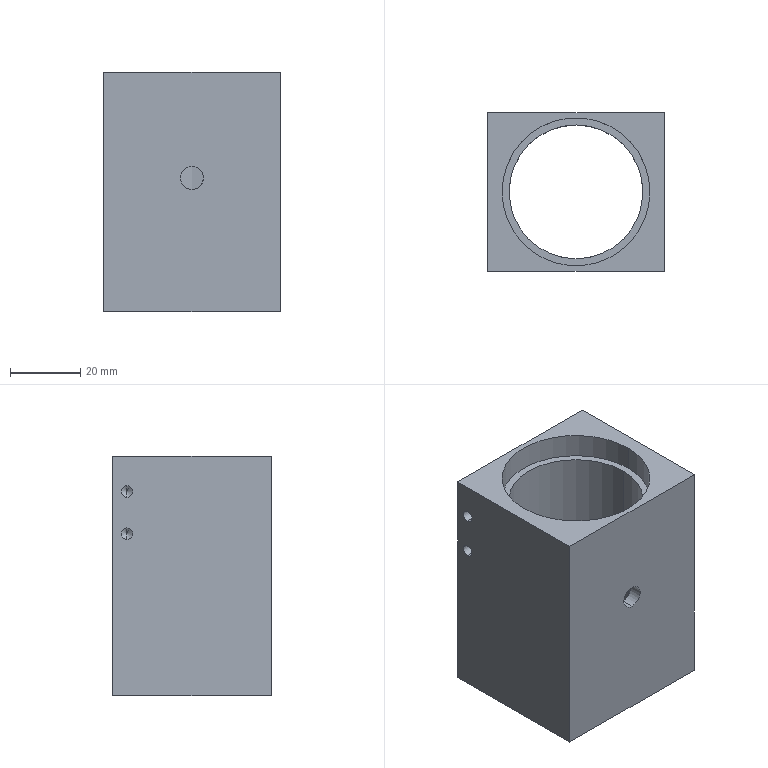Part | SolidWorks | features HoleWzd 4, Cut 2, Extrusion 1, ICE 1 | 1 solid | 48 faces | box 50 x 45 x 68 mm | volume 67005 mm3 | cylinder 24 | cone 16 | plane 8 | commonest cylinder face diameters 3.3 x16 42 x4 6.5 x2 38 x2
STEP:
#1=CARTESIAN_POINT('',(6.65,36.5,10.1));
#2=VERTEX_POINT('',#1);
#3=CARTESIAN_POINT('',(3.35,36.5,10.1));
#4=VERTEX_POINT('',#3);
#5=CARTESIAN_POINT('',(5.,36.5,10.1));
#6=DIRECTION('',(0.,0.,-1.));
#7=DIRECTION('',(-1.,0.,0.));
#8=AXIS2_PLACEMENT_3D('',#5,#6,#7);
#9=CIRCLE('',#8,1.65);
#10=EDGE_CURVE('',#2,#4,#9,.T.);
#11=ORIENTED_EDGE('',*,*,#10,.F.);
#12=CARTESIAN_POINT('',(6.65,36.5,0.));
#13=VERTEX_POINT('',#12);
#14=CARTESIAN_POINT('',(6.65,36.5,0.));
#15=DIRECTION('',(0.,0.,-1.));
#16=VECTOR('',#15,1000.);
#17=LINE('',#14,#16);
#18=EDGE_CURVE('',#2,#13,#17,.T.);
#19=ORIENTED_EDGE('',*,*,#18,.T.);
#20=CARTESIAN_POINT('',(3.35,36.5,0.));
#21=VERTEX_POINT('',#20);
#22=CARTESIAN_POINT('',(5.,36.5,0.));
#23=DIRECTION('',(0.,0.,-1.));
#24=DIRECTION('',(-1.,0.,0.));
#25=AXIS2_PLACEMENT_3D('',#22,#23,#24);
#26=CIRCLE('',#25,1.65);
#27=EDGE_CURVE('',#13,#21,#26,.T.);
#28=ORIENTED_EDGE('',*,*,#27,.T.);
#29=CARTESIAN_POINT('',(3.35,36.5,0.));
#30=DIRECTION('',(0.,0.,-1.));
#31=VECTOR('',#30,1000.);
#32=LINE('',#29,#31);
#33=EDGE_CURVE('',#4,#21,#32,.T.);
#34=ORIENTED_EDGE('',*,*,#33,.F.);
#35=EDGE_LOOP('',(#11,#19,#28,#34));
#36=FACE_OUTER_BOUND('',#35,.T.);
#37=CARTESIAN_POINT('',(5.,36.5,0.));
#38=DIRECTION('',(0.,0.,-1.));
#39=DIRECTION('',(-1.,0.,0.));
#40=AXIS2_PLACEMENT_3D('',#37,#38,#39);
#41=CYLINDRICAL_SURFACE('',#40,1.65);
#42=ADVANCED_FACE('',(#36),#41,.F.);
#43=CARTESIAN_POINT('',(5.,36.5,11.091));
#44=VERTEX_POINT('',#43);
#45=CARTESIAN_POINT('',(3.35,36.5,10.1));
#46=DIRECTION('',(-0.8572,0.,-0.515));
#47=VECTOR('',#46,1000.);
#48=LINE('',#45,#47);
#49=EDGE_CURVE('',#44,#4,#48,.T.);
#50=ORIENTED_EDGE('',*,*,#49,.F.);
#51=CARTESIAN_POINT('',(6.65,36.5,10.1));
#52=DIRECTION('',(0.8572,0.,-0.515));
#53=VECTOR('',#52,1000.);
#54=LINE('',#51,#53);
#55=EDGE_CURVE('',#44,#2,#54,.T.);
#56=ORIENTED_EDGE('',*,*,#55,.T.);
#57=ORIENTED_EDGE('',*,*,#10,.T.);
#58=EDGE_LOOP('',(#50,#56,#57));
#59=FACE_OUTER_BOUND('',#58,.T.);
#60=CARTESIAN_POINT('',(5.,36.5,10.1));
#61=DIRECTION('',(0.,0.,-1.));
#62=DIRECTION('',(-1.,0.,0.));
#63=AXIS2_PLACEMENT_3D('',#60,#61,#62);
#64=CONICAL_SURFACE('',#63,1.65,1.03);
#65=ADVANCED_FACE('',(#59),#64,.F.);
#66=CARTESIAN_POINT('',(46.65,36.5,10.1));
#67=VERTEX_POINT('',#66);
#68=CARTESIAN_POINT('',(43.35,36.5,10.1));
#69=VERTEX_POINT('',#68);
#70=CARTESIAN_POINT('',(45.,36.5,10.1));
#71=DIRECTION('',(0.,0.,-1.));
#72=DIRECTION('',(-1.,0.,0.));
#73=AXIS2_PLACEMENT_3D('',#70,#71,#72);
#74=CIRCLE('',#73,1.65);
#75=EDGE_CURVE('',#67,#69,#74,.T.);
#76=ORIENTED_EDGE('',*,*,#75,.F.);
#77=CARTESIAN_POINT('',(46.65,36.5,0.));
#78=VERTEX_POINT('',#77);
#79=CARTESIAN_POINT('',(46.65,36.5,0.));
#80=DIRECTION('',(0.,0.,-1.));
#81=VECTOR('',#80,1000.);
#82=LINE('',#79,#81);
#83=EDGE_CURVE('',#67,#78,#82,.T.);
#84=ORIENTED_EDGE('',*,*,#83,.T.);
#85=CARTESIAN_POINT('',(43.35,36.5,0.));
#86=VERTEX_POINT('',#85);
#87=CARTESIAN_POINT('',(45.,36.5,0.));
#88=DIRECTION('',(0.,0.,-1.));
#89=DIRECTION('',(-1.,0.,0.));
#90=AXIS2_PLACEMENT_3D('',#87,#88,#89);
#91=CIRCLE('',#90,1.65);
#92=EDGE_CURVE('',#78,#86,#91,.T.);
#93=ORIENTED_EDGE('',*,*,#92,.T.);
#94=CARTESIAN_POINT('',(43.35,36.5,0.));
#95=DIRECTION('',(0.,0.,-1.));
#96=VECTOR('',#95,1000.);
#97=LINE('',#94,#96);
#98=EDGE_CURVE('',#69,#86,#97,.T.);
#99=ORIENTED_EDGE('',*,*,#98,.F.);
#100=EDGE_LOOP('',(#76,#84,#93,#99));
#101=FACE_OUTER_BOUND('',#100,.T.);
#102=CARTESIAN_POINT('',(45.,36.5,0.));
#103=DIRECTION('',(0.,0.,-1.));
#104=DIRECTION('',(-1.,0.,0.));
#105=AXIS2_PLACEMENT_3D('',#102,#103,#104);
#106=CYLINDRICAL_SURFACE('',#105,1.65);
#107=ADVANCED_FACE('',(#101),#106,.F.);
#108=CARTESIAN_POINT('',(45.,36.5,11.091));
#109=VERTEX_POINT('',#108);
#110=CARTESIAN_POINT('',(43.35,36.5,10.1));
#111=DIRECTION('',(-0.8572,0.,-0.515));
#112=VECTOR('',#111,1000.);
#113=LINE('',#110,#112);
#114=EDGE_CURVE('',#109,#69,#113,.T.);
#115=ORIENTED_EDGE('',*,*,#114,.F.);
#116=CARTESIAN_POINT('',(46.65,36.5,10.1));
#117=DIRECTION('',(0.8572,0.,-0.515));
#118=VECTOR('',#117,1000.);
#119=LINE('',#116,#118);
#120=EDGE_CURVE('',#109,#67,#119,.T.);
#121=ORIENTED_EDGE('',*,*,#120,.T.);
#122=ORIENTED_EDGE('',*,*,#75,.T.);
#123=EDGE_LOOP('',(#115,#121,#122));
#124=FACE_OUTER_BOUND('',#123,.T.);
#125=CARTESIAN_POINT('',(45.,36.5,10.1));
#126=DIRECTION('',(0.,0.,-1.));
#127=DIRECTION('',(-1.,0.,0.));
#128=AXIS2_PLACEMENT_3D('',#125,#126,#127);
#129=CONICAL_SURFACE('',#128,1.65,1.03);
#130=ADVANCED_FACE('',(#124),#129,.F.);
#131=CARTESIAN_POINT('',(46.65,8.5,10.1));
#132=VERTEX_POINT('',#131);
#133=CARTESIAN_POINT('',(43.35,8.5,10.1));
#134=VERTEX_POINT('',#133);
#135=CARTESIAN_POINT('',(45.,8.5,10.1));
#136=DIRECTION('',(0.,0.,-1.));
#137=DIRECTION('',(-1.,0.,0.));
#138=AXIS2_PLACEMENT_3D('',#135,#136,#137);
#139=CIRCLE('',#138,1.65);
#140=EDGE_CURVE('',#132,#134,#139,.T.);
#141=ORIENTED_EDGE('',*,*,#140,.F.);
#142=CARTESIAN_POINT('',(46.65,8.5,0.));
#143=VERTEX_POINT('',#142);
#144=CARTESIAN_POINT('',(46.65,8.5,0.));
#145=DIRECTION('',(0.,0.,-1.));
#146=VECTOR('',#145,1000.);
#147=LINE('',#144,#146);
#148=EDGE_CURVE('',#132,#143,#147,.T.);
#149=ORIENTED_EDGE('',*,*,#148,.T.);
#150=CARTESIAN_POINT('',(43.35,8.5,0.));
#151=VERTEX_POINT('',#150);
#152=CARTESIAN_POINT('',(45.,8.5,0.));
#153=DIRECTION('',(0.,0.,-1.));
#154=DIRECTION('',(-1.,0.,0.));
#155=AXIS2_PLACEMENT_3D('',#152,#153,#154);
#156=CIRCLE('',#155,1.65);
#157=EDGE_CURVE('',#143,#151,#156,.T.);
#158=ORIENTED_EDGE('',*,*,#157,.T.);
#159=CARTESIAN_POINT('',(43.35,8.5,0.));
#160=DIRECTION('',(0.,0.,-1.));
#161=VECTOR('',#160,1000.);
#162=LINE('',#159,#161);
#163=EDGE_CURVE('',#134,#151,#162,.T.);
#164=ORIENTED_EDGE('',*,*,#163,.F.);
#165=EDGE_LOOP('',(#141,#149,#158,#164));
#166=FACE_OUTER_BOUND('',#165,.T.);
#167=CARTESIAN_POINT('',(45.,8.5,0.));
#168=DIRECTION('',(0.,0.,-1.));
#169=DIRECTION('',(-1.,0.,0.));
#170=AXIS2_PLACEMENT_3D('',#167,#168,#169);
#171=CYLINDRICAL_SURFACE('',#170,1.65);
#172=ADVANCED_FACE('',(#166),#171,.F.);
#173=CARTESIAN_POINT('',(45.,8.5,11.091));
#174=VERTEX_POINT('',#173);
#175=CARTESIAN_POINT('',(43.35,8.5,10.1));
#176=DIRECTION('',(-0.8572,0.,-0.515));
#177=VECTOR('',#176,1000.);
#178=LINE('',#175,#177);
#179=EDGE_CURVE('',#174,#134,#178,.T.);
#180=ORIENTED_EDGE('',*,*,#179,.F.);
#181=CARTESIAN_POINT('',(46.65,8.5,10.1));
#182=DIRECTION('',(0.8572,0.,-0.515));
#183=VECTOR('',#182,1000.);
#184=LINE('',#181,#183);
#185=EDGE_CURVE('',#174,#132,#184,.T.);
#186=ORIENTED_EDGE('',*,*,#185,.T.);
#187=ORIENTED_EDGE('',*,*,#140,.T.);
#188=EDGE_LOOP('',(#180,#186,#187));
#189=FACE_OUTER_BOUND('',#188,.T.);
#190=CARTESIAN_POINT('',(45.,8.5,10.1));
#191=DIRECTION('',(0.,0.,-1.));
#192=DIRECTION('',(-1.,0.,0.));
#193=AXIS2_PLACEMENT_3D('',#190,#191,#192);
#194=CONICAL_SURFACE('',#193,1.65,1.03);
#195=ADVANCED_FACE('',(#189),#194,.F.);
#196=CARTESIAN_POINT('',(6.65,8.5,10.1));
#197=VERTEX_POINT('',#196);
#198=CARTESIAN_POINT('',(3.35,8.5,10.1));
#199=VERTEX_POINT('',#198);
#200=CARTESIAN_POINT('',(5.,8.5,10.1));
#201=DIRECTION('',(0.,0.,-1.));
#202=DIRECTION('',(-1.,0.,0.));
#203=AXIS2_PLACEMENT_3D('',#200,#201,#202);
#204=CIRCLE('',#203,1.65);
#205=EDGE_CURVE('',#197,#199,#204,.T.);
#206=ORIENTED_EDGE('',*,*,#205,.F.);
#207=CARTESIAN_POINT('',(6.65,8.5,0.));
#208=VERTEX_POINT('',#207);
#209=CARTESIAN_POINT('',(6.65,8.5,0.));
#210=DIRECTION('',(0.,0.,-1.));
#211=VECTOR('',#210,1000.);
#212=LINE('',#209,#211);
#213=EDGE_CURVE('',#197,#208,#212,.T.);
#214=ORIENTED_EDGE('',*,*,#213,.T.);
#215=CARTESIAN_POINT('',(3.35,8.5,0.));
#216=VERTEX_POINT('',#215);
#217=CARTESIAN_POINT('',(5.,8.5,0.));
#218=DIRECTION('',(0.,0.,-1.));
#219=DIRECTION('',(-1.,0.,0.));
#220=AXIS2_PLACEMENT_3D('',#217,#218,#219);
#221=CIRCLE('',#220,1.65);
#222=EDGE_CURVE('',#208,#216,#221,.T.);
#223=ORIENTED_EDGE('',*,*,#222,.T.);
#224=CARTESIAN_POINT('',(3.35,8.5,0.));
#225=DIRECTION('',(0.,0.,-1.));
#226=VECTOR('',#225,1000.);
#227=LINE('',#224,#226);
#228=EDGE_CURVE('',#199,#216,#227,.T.);
#229=ORIENTED_EDGE('',*,*,#228,.F.);
#230=EDGE_LOOP('',(#206,#214,#223,#229));
#231=FACE_OUTER_BOUND('',#230,.T.);
#232=CARTESIAN_POINT('',(5.,8.5,0.));
#233=DIRECTION('',(0.,0.,-1.));
#234=DIRECTION('',(-1.,0.,0.));
#235=AXIS2_PLACEMENT_3D('',#232,#233,#234);
#236=CYLINDRICAL_SURFACE('',#235,1.65);
#237=ADVANCED_FACE('',(#231),#236,.F.);
#238=CARTESIAN_POINT('',(5.,8.5,11.091));
#239=VERTEX_POINT('',#238);
#240=CARTESIAN_POINT('',(3.35,8.5,10.1));
#241=DIRECTION('',(-0.8572,0.,-0.515));
#242=VECTOR('',#241,1000.);
#243=LINE('',#240,#242);
#244=EDGE_CURVE('',#239,#199,#243,.T.);
#245=ORIENTED_EDGE('',*,*,#244,.F.);
#246=CARTESIAN_POINT('',(6.65,8.5,10.1));
#247=DIRECTION('',(0.8572,0.,-0.515));
#248=VECTOR('',#247,1000.);
#249=LINE('',#246,#248);
#250=EDGE_CURVE('',#239,#197,#249,.T.);
#251=ORIENTED_EDGE('',*,*,#250,.T.);
#252=ORIENTED_EDGE('',*,*,#205,.T.);
#253=EDGE_LOOP('',(#245,#251,#252));
#254=FACE_OUTER_BOUND('',#253,.T.);
#255=CARTESIAN_POINT('',(5.,8.5,10.1));
#256=DIRECTION('',(0.,0.,-1.));
#257=DIRECTION('',(-1.,0.,0.));
#258=AXIS2_PLACEMENT_3D('',#255,#256,#257);
#259=CONICAL_SURFACE('',#258,1.65,1.03);
#260=ADVANCED_FACE('',(#254),#259,.F.);
#261=CARTESIAN_POINT('',(25.,3.5,41.25));
#262=VERTEX_POINT('',#261);
#263=CARTESIAN_POINT('',(25.,3.5,34.75));
#264=VERTEX_POINT('',#263);
#265=CARTESIAN_POINT('',(25.,3.5,41.25));
#266=CARTESIAN_POINT('',(24.788,3.5,41.25));
#267=CARTESIAN_POINT('',(24.576,3.504,41.229));
#268=CARTESIAN_POINT('',(24.156,3.518,41.146));
#269=CARTESIAN_POINT('',(23.952,3.528,41.084));
#270=CARTESIAN_POINT('',(23.56,3.554,40.921));
#271=CARTESIAN_POINT('',(23.371,3.569,40.82));
#272=CARTESIAN_POINT('',(23.017,3.603,40.583));
#273=CARTESIAN_POINT('',(22.853,3.621,40.449));
#274=CARTESIAN_POINT('',(22.553,3.658,40.15));
#275=CARTESIAN_POINT('',(22.416,3.676,39.983));
#276=CARTESIAN_POINT('',(22.181,3.71,39.631));
#277=CARTESIAN_POINT('',(22.081,3.725,39.444));
#278=CARTESIAN_POINT('',(21.917,3.752,39.05));
#279=CARTESIAN_POINT('',(21.854,3.762,38.845));
#280=CARTESIAN_POINT('',(21.771,3.776,38.429));
#281=CARTESIAN_POINT('',(21.75,3.78,38.217));
#282=CARTESIAN_POINT('',(21.75,3.78,37.787));
#283=CARTESIAN_POINT('',(21.771,3.776,37.576));
#284=CARTESIAN_POINT('',(21.853,3.762,37.16));
#285=CARTESIAN_POINT('',(21.916,3.752,36.953));
#286=CARTESIAN_POINT('',(22.079,3.726,36.56));
#287=CARTESIAN_POINT('',(22.178,3.71,36.373));
#288=CARTESIAN_POINT('',(22.414,3.676,36.02));
#289=CARTESIAN_POINT('',(22.551,3.658,35.853));
#290=CARTESIAN_POINT('',(22.85,3.621,35.554));
#291=CARTESIAN_POINT('',(23.013,3.603,35.419));
#292=CARTESIAN_POINT('',(23.369,3.569,35.181));
#293=CARTESIAN_POINT('',(23.556,3.554,35.081));
#294=CARTESIAN_POINT('',(23.947,3.528,34.918));
#295=CARTESIAN_POINT('',(24.153,3.518,34.855));
#296=CARTESIAN_POINT('',(24.572,3.504,34.771));
#297=CARTESIAN_POINT('',(24.785,3.5,34.75));
#298=CARTESIAN_POINT('',(25.,3.5,34.75));
#299=B_SPLINE_CURVE_WITH_KNOTS('',3,(#265,#266,#267,#268,#269,#270,#271,#272,#273,#274,#275,#276,#277,#278,#279,#280,#281,#282,#283,#284,#285,#286,#287,#288,#289,#290,#291,#292,#293,#294,#295,#296,#297,#298),.UNSPECIFIED.,.F.,.F.,(4,2,2,2,2,2,2,2,2,2,2,2,2,2,2,2,4),(0.01018,0.01082,0.01145,0.01209,0.01272,0.01336,0.014,0.01463,0.01527,0.0159,0.01654,0.01718,0.01781,0.01845,0.01908,0.01972,0.02036),.UNSPECIFIED.);
#300=EDGE_CURVE('',#262,#264,#299,.T.);
#301=ORIENTED_EDGE('',*,*,#300,.F.);
#302=CARTESIAN_POINT('',(25.,0.,41.25));
#303=VERTEX_POINT('',#302);
#304=CARTESIAN_POINT('',(25.,0.,41.25));
#305=DIRECTION('',(0.,-1.,0.));
#306=VECTOR('',#305,1000.);
#307=LINE('',#304,#306);
#308=EDGE_CURVE('',#262,#303,#307,.T.);
#309=ORIENTED_EDGE('',*,*,#308,.T.);
#310=CARTESIAN_POINT('',(25.,0.,34.75));
#311=VERTEX_POINT('',#310);
#312=CARTESIAN_POINT('',(25.,0.,38.));
#313=DIRECTION('',(0.,-1.,0.));
#314=DIRECTION('',(0.,0.,-1.));
#315=AXIS2_PLACEMENT_3D('',#312,#313,#314);
#316=CIRCLE('',#315,3.25);
#317=EDGE_CURVE('',#303,#311,#316,.T.);
#318=ORIENTED_EDGE('',*,*,#317,.T.);
#319=CARTESIAN_POINT('',(25.,0.,34.75));
#320=DIRECTION('',(0.,-1.,0.));
#321=VECTOR('',#320,1000.);
#322=LINE('',#319,#321);
#323=EDGE_CURVE('',#264,#311,#322,.T.);
#324=ORIENTED_EDGE('',*,*,#323,.F.);
#325=EDGE_LOOP('',(#301,#309,#318,#324));
#326=FACE_OUTER_BOUND('',#325,.T.);
#327=CARTESIAN_POINT('',(25.,0.,38.));
#328=DIRECTION('',(0.,-1.,0.));
#329=DIRECTION('',(0.,0.,-1.));
#330=AXIS2_PLACEMENT_3D('',#327,#328,#329);
#331=CYLINDRICAL_SURFACE('',#330,3.25);
#332=ADVANCED_FACE('',(#326),#331,.F.);
#333=CARTESIAN_POINT('',(10.1,41.,44.35));
#334=VERTEX_POINT('',#333);
#335=CARTESIAN_POINT('',(10.1,41.,47.65));
#336=VERTEX_POINT('',#335);
#337=CARTESIAN_POINT('',(10.1,41.,46.));
#338=DIRECTION('',(-1.,0.,0.));
#339=DIRECTION('',(0.,0.,1.));
#340=AXIS2_PLACEMENT_3D('',#337,#338,#339);
#341=CIRCLE('',#340,1.65);
#342=EDGE_CURVE('',#334,#336,#341,.T.);
#343=ORIENTED_EDGE('',*,*,#342,.F.);
#344=CARTESIAN_POINT('',(0.,41.,44.35));
#345=VERTEX_POINT('',#344);
#346=CARTESIAN_POINT('',(0.,41.,44.35));
#347=DIRECTION('',(-1.,0.,0.));
#348=VECTOR('',#347,1000.);
#349=LINE('',#346,#348);
#350=EDGE_CURVE('',#334,#345,#349,.T.);
#351=ORIENTED_EDGE('',*,*,#350,.T.);
#352=CARTESIAN_POINT('',(0.,41.,47.65));
#353=VERTEX_POINT('',#352);
#354=CARTESIAN_POINT('',(0.,41.,46.));
#355=DIRECTION('',(-1.,0.,0.));
#356=DIRECTION('',(0.,0.,1.));
#357=AXIS2_PLACEMENT_3D('',#354,#355,#356);
#358=CIRCLE('',#357,1.65);
#359=EDGE_CURVE('',#345,#353,#358,.T.);
#360=ORIENTED_EDGE('',*,*,#359,.T.);
#361=CARTESIAN_POINT('',(0.,41.,47.65));
#362=DIRECTION('',(-1.,0.,0.));
#363=VECTOR('',#362,1000.);
#364=LINE('',#361,#363);
#365=EDGE_CURVE('',#336,#353,#364,.T.);
#366=ORIENTED_EDGE('',*,*,#365,.F.);
#367=EDGE_LOOP('',(#343,#351,#360,#366));
#368=FACE_OUTER_BOUND('',#367,.T.);
#369=CARTESIAN_POINT('',(0.,41.,46.));
#370=DIRECTION('',(-1.,0.,0.));
#371=DIRECTION('',(0.,0.,1.));
#372=AXIS2_PLACEMENT_3D('',#369,#370,#371);
#373=CYLINDRICAL_SURFACE('',#372,1.65);
#374=ADVANCED_FACE('',(#368),#373,.F.);
#375=CARTESIAN_POINT('',(11.091,41.,46.));
#376=VERTEX_POINT('',#375);
#377=CARTESIAN_POINT('',(10.1,41.,47.65));
#378=DIRECTION('',(-0.515,0.,0.8572));
#379=VECTOR('',#378,1000.);
#380=LINE('',#377,#379);
#381=EDGE_CURVE('',#376,#336,#380,.T.);
#382=ORIENTED_EDGE('',*,*,#381,.F.);
#383=CARTESIAN_POINT('',(10.1,41.,44.35));
#384=DIRECTION('',(-0.515,0.,-0.8572));
#385=VECTOR('',#384,1000.);
#386=LINE('',#383,#385);
#387=EDGE_CURVE('',#376,#334,#386,.T.);
#388=ORIENTED_EDGE('',*,*,#387,.T.);
#389=ORIENTED_EDGE('',*,*,#342,.T.);
#390=EDGE_LOOP('',(#382,#388,#389));
#391=FACE_OUTER_BOUND('',#390,.T.);
#392=CARTESIAN_POINT('',(10.1,41.,46.));
#393=DIRECTION('',(-1.,0.,0.));
#394=DIRECTION('',(0.,0.,1.));
#395=AXIS2_PLACEMENT_3D('',#392,#393,#394);
#396=CONICAL_SURFACE('',#395,1.65,1.03);
#397=ADVANCED_FACE('',(#391),#396,.F.);
#398=CARTESIAN_POINT('',(10.1,41.,56.35));
#399=VERTEX_POINT('',#398);
#400=CARTESIAN_POINT('',(10.1,41.,59.65));
#401=VERTEX_POINT('',#400);
#402=CARTESIAN_POINT('',(10.1,41.,58.));
#403=DIRECTION('',(-1.,0.,0.));
#404=DIRECTION('',(0.,0.,1.));
#405=AXIS2_PLACEMENT_3D('',#402,#403,#404);
#406=CIRCLE('',#405,1.65);
#407=EDGE_CURVE('',#399,#401,#406,.T.);
#408=ORIENTED_EDGE('',*,*,#407,.F.);
#409=CARTESIAN_POINT('',(0.,41.,56.35));
#410=VERTEX_POINT('',#409);
#411=CARTESIAN_POINT('',(0.,41.,56.35));
#412=DIRECTION('',(-1.,0.,0.));
#413=VECTOR('',#412,1000.);
#414=LINE('',#411,#413);
#415=EDGE_CURVE('',#399,#410,#414,.T.);
#416=ORIENTED_EDGE('',*,*,#415,.T.);
#417=CARTESIAN_POINT('',(0.,41.,59.65));
#418=VERTEX_POINT('',#417);
#419=CARTESIAN_POINT('',(0.,41.,58.));
#420=DIRECTION('',(-1.,0.,0.));
#421=DIRECTION('',(0.,0.,1.));
#422=AXIS2_PLACEMENT_3D('',#419,#420,#421);
#423=CIRCLE('',#422,1.65);
#424=EDGE_CURVE('',#410,#418,#423,.T.);
#425=ORIENTED_EDGE('',*,*,#424,.T.);
#426=CARTESIAN_POINT('',(0.,41.,59.65));
#427=DIRECTION('',(-1.,0.,0.));
#428=VECTOR('',#427,1000.);
#429=LINE('',#426,#428);
#430=EDGE_CURVE('',#401,#418,#429,.T.);
#431=ORIENTED_EDGE('',*,*,#430,.F.);
#432=EDGE_LOOP('',(#408,#416,#425,#431));
#433=FACE_OUTER_BOUND('',#432,.T.);
#434=CARTESIAN_POINT('',(0.,41.,58.));
#435=DIRECTION('',(-1.,0.,0.));
#436=DIRECTION('',(0.,0.,1.));
#437=AXIS2_PLACEMENT_3D('',#434,#435,#436);
#438=CYLINDRICAL_SURFACE('',#437,1.65);
#439=ADVANCED_FACE('',(#433),#438,.F.);
#440=CARTESIAN_POINT('',(11.091,41.,58.));
#441=VERTEX_POINT('',#440);
#442=CARTESIAN_POINT('',(10.1,41.,59.65));
#443=DIRECTION('',(-0.515,0.,0.8572));
#444=VECTOR('',#443,1000.);
#445=LINE('',#442,#444);
#446=EDGE_CURVE('',#441,#401,#445,.T.);
#447=ORIENTED_EDGE('',*,*,#446,.F.);
#448=CARTESIAN_POINT('',(10.1,41.,56.35));
#449=DIRECTION('',(-0.515,0.,-0.8572));
#450=VECTOR('',#449,1000.);
#451=LINE('',#448,#450);
#452=EDGE_CURVE('',#441,#399,#451,.T.);
#453=ORIENTED_EDGE('',*,*,#452,.T.);
#454=ORIENTED_EDGE('',*,*,#407,.T.);
#455=EDGE_LOOP('',(#447,#453,#454));
#456=FACE_OUTER_BOUND('',#455,.T.);
#457=CARTESIAN_POINT('',(10.1,41.,58.));
#458=DIRECTION('',(-1.,0.,0.));
#459=DIRECTION('',(0.,0.,1.));
#460=AXIS2_PLACEMENT_3D('',#457,#458,#459);
#461=CONICAL_SURFACE('',#460,1.65,1.03);
#462=ADVANCED_FACE('',(#456),#461,.F.);
#463=CARTESIAN_POINT('',(39.9,41.,59.65));
#464=VERTEX_POINT('',#463);
#465=CARTESIAN_POINT('',(39.9,41.,56.35));
#466=VERTEX_POINT('',#465);
#467=CARTESIAN_POINT('',(39.9,41.,58.));
#468=DIRECTION('',(1.,0.,0.));
#469=DIRECTION('',(0.,0.,-1.));
#470=AXIS2_PLACEMENT_3D('',#467,#468,#469);
#471=CIRCLE('',#470,1.65);
#472=EDGE_CURVE('',#464,#466,#471,.T.);
#473=ORIENTED_EDGE('',*,*,#472,.F.);
#474=CARTESIAN_POINT('',(50.,41.,59.65));
#475=VERTEX_POINT('',#474);
#476=CARTESIAN_POINT('',(50.,41.,59.65));
#477=DIRECTION('',(1.,0.,0.));
#478=VECTOR('',#477,1000.);
#479=LINE('',#476,#478);
#480=EDGE_CURVE('',#464,#475,#479,.T.);
#481=ORIENTED_EDGE('',*,*,#480,.T.);
#482=CARTESIAN_POINT('',(50.,41.,56.35));
#483=VERTEX_POINT('',#482);
#484=CARTESIAN_POINT('',(50.,41.,58.));
#485=DIRECTION('',(1.,0.,0.));
#486=DIRECTION('',(0.,0.,-1.));
#487=AXIS2_PLACEMENT_3D('',#484,#485,#486);
#488=CIRCLE('',#487,1.65);
#489=EDGE_CURVE('',#475,#483,#488,.T.);
#490=ORIENTED_EDGE('',*,*,#489,.T.);
#491=CARTESIAN_POINT('',(50.,41.,56.35));
#492=DIRECTION('',(1.,0.,0.));
#493=VECTOR('',#492,1000.);
#494=LINE('',#491,#493);
#495=EDGE_CURVE('',#466,#483,#494,.T.);
#496=ORIENTED_EDGE('',*,*,#495,.F.);
#497=EDGE_LOOP('',(#473,#481,#490,#496));
#498=FACE_OUTER_BOUND('',#497,.T.);
#499=CARTESIAN_POINT('',(50.,41.,58.));
#500=DIRECTION('',(1.,0.,0.));
#501=DIRECTION('',(0.,0.,-1.));
#502=AXIS2_PLACEMENT_3D('',#499,#500,#501);
#503=CYLINDRICAL_SURFACE('',#502,1.65);
#504=ADVANCED_FACE('',(#498),#503,.F.);
#505=CARTESIAN_POINT('',(38.909,41.,58.));
#506=VERTEX_POINT('',#505);
#507=CARTESIAN_POINT('',(39.9,41.,56.35));
#508=DIRECTION('',(0.515,0.,-0.8572));
#509=VECTOR('',#508,1000.);
#510=LINE('',#507,#509);
#511=EDGE_CURVE('',#506,#466,#510,.T.);
#512=ORIENTED_EDGE('',*,*,#511,.F.);
#513=CARTESIAN_POINT('',(39.9,41.,59.65));
#514=DIRECTION('',(0.515,0.,0.8572));
#515=VECTOR('',#514,1000.);
#516=LINE('',#513,#515);
#517=EDGE_CURVE('',#506,#464,#516,.T.);
#518=ORIENTED_EDGE('',*,*,#517,.T.);
#519=ORIENTED_EDGE('',*,*,#472,.T.);
#520=EDGE_LOOP('',(#512,#518,#519));
#521=FACE_OUTER_BOUND('',#520,.T.);
#522=CARTESIAN_POINT('',(39.9,41.,58.));
#523=DIRECTION('',(1.,0.,0.));
#524=DIRECTION('',(0.,0.,-1.));
#525=AXIS2_PLACEMENT_3D('',#522,#523,#524);
#526=CONICAL_SURFACE('',#525,1.65,1.03);
#527=ADVANCED_FACE('',(#521),#526,.F.);
#528=CARTESIAN_POINT('',(39.9,41.,47.65));
#529=VERTEX_POINT('',#528);
#530=CARTESIAN_POINT('',(39.9,41.,44.35));
#531=VERTEX_POINT('',#530);
#532=CARTESIAN_POINT('',(39.9,41.,46.));
#533=DIRECTION('',(1.,0.,0.));
#534=DIRECTION('',(0.,0.,-1.));
#535=AXIS2_PLACEMENT_3D('',#532,#533,#534);
#536=CIRCLE('',#535,1.65);
#537=EDGE_CURVE('',#529,#531,#536,.T.);
#538=ORIENTED_EDGE('',*,*,#537,.F.);
#539=CARTESIAN_POINT('',(50.,41.,47.65));
#540=VERTEX_POINT('',#539);
#541=CARTESIAN_POINT('',(50.,41.,47.65));
#542=DIRECTION('',(1.,0.,0.));
#543=VECTOR('',#542,1000.);
#544=LINE('',#541,#543);
#545=EDGE_CURVE('',#529,#540,#544,.T.);
#546=ORIENTED_EDGE('',*,*,#545,.T.);
#547=CARTESIAN_POINT('',(50.,41.,44.35));
#548=VERTEX_POINT('',#547);
#549=CARTESIAN_POINT('',(50.,41.,46.));
#550=DIRECTION('',(1.,0.,0.));
#551=DIRECTION('',(0.,0.,-1.));
#552=AXIS2_PLACEMENT_3D('',#549,#550,#551);
#553=CIRCLE('',#552,1.65);
#554=EDGE_CURVE('',#540,#548,#553,.T.);
#555=ORIENTED_EDGE('',*,*,#554,.T.);
#556=CARTESIAN_POINT('',(50.,41.,44.35));
#557=DIRECTION('',(1.,0.,0.));
#558=VECTOR('',#557,1000.);
#559=LINE('',#556,#558);
#560=EDGE_CURVE('',#531,#548,#559,.T.);
#561=ORIENTED_EDGE('',*,*,#560,.F.);
#562=EDGE_LOOP('',(#538,#546,#555,#561));
#563=FACE_OUTER_BOUND('',#562,.T.);
#564=CARTESIAN_POINT('',(50.,41.,46.));
#565=DIRECTION('',(1.,0.,0.));
#566=DIRECTION('',(0.,0.,-1.));
#567=AXIS2_PLACEMENT_3D('',#564,#565,#566);
#568=CYLINDRICAL_SURFACE('',#567,1.65);
#569=ADVANCED_FACE('',(#563),#568,.F.);
#570=CARTESIAN_POINT('',(38.909,41.,46.));
#571=VERTEX_POINT('',#570);
#572=CARTESIAN_POINT('',(39.9,41.,44.35));
#573=DIRECTION('',(0.515,0.,-0.8572));
#574=VECTOR('',#573,1000.);
#575=LINE('',#572,#574);
#576=EDGE_CURVE('',#571,#531,#575,.T.);
#577=ORIENTED_EDGE('',*,*,#576,.F.);
#578=CARTESIAN_POINT('',(39.9,41.,47.65));
#579=DIRECTION('',(0.515,0.,0.8572));
#580=VECTOR('',#579,1000.);
#581=LINE('',#578,#580);
#582=EDGE_CURVE('',#571,#529,#581,.T.);
#583=ORIENTED_EDGE('',*,*,#582,.T.);
#584=ORIENTED_EDGE('',*,*,#537,.T.);
#585=EDGE_LOOP('',(#577,#583,#584));
#586=FACE_OUTER_BOUND('',#585,.T.);
#587=CARTESIAN_POINT('',(39.9,41.,46.));
#588=DIRECTION('',(1.,0.,0.));
#589=DIRECTION('',(0.,0.,-1.));
#590=AXIS2_PLACEMENT_3D('',#587,#588,#589);
#591=CONICAL_SURFACE('',#590,1.65,1.03);
#592=ADVANCED_FACE('',(#586),#591,.F.);
#593=CARTESIAN_POINT('',(46.,22.5,25.));
#594=VERTEX_POINT('',#593);
#595=CARTESIAN_POINT('',(4.,22.5,25.));
#596=VERTEX_POINT('',#595);
#597=CARTESIAN_POINT('',(25.,22.5,25.));
#598=DIRECTION('',(0.,0.,-1.));
#599=DIRECTION('',(-1.,0.,0.));
#600=AXIS2_PLACEMENT_3D('',#597,#598,#599);
#601=CIRCLE('',#600,21.);
#602=EDGE_CURVE('',#594,#596,#601,.T.);
#603=ORIENTED_EDGE('',*,*,#602,.F.);
#604=CARTESIAN_POINT('',(46.,22.5,0.));
#605=VERTEX_POINT('',#604);
#606=CARTESIAN_POINT('',(46.,22.5,25.));
#607=DIRECTION('',(0.,0.,-1.));
#608=VECTOR('',#607,1000.);
#609=LINE('',#606,#608);
#610=EDGE_CURVE('',#594,#605,#609,.T.);
#611=ORIENTED_EDGE('',*,*,#610,.T.);
#612=CARTESIAN_POINT('',(4.,22.5,0.));
#613=VERTEX_POINT('',#612);
#614=CARTESIAN_POINT('',(25.,22.5,0.));
#615=DIRECTION('',(0.,0.,-1.));
#616=DIRECTION('',(-1.,0.,0.));
#617=AXIS2_PLACEMENT_3D('',#614,#615,#616);
#618=CIRCLE('',#617,21.);
#619=EDGE_CURVE('',#605,#613,#618,.T.);
#620=ORIENTED_EDGE('',*,*,#619,.T.);
#621=CARTESIAN_POINT('',(4.,22.5,25.));
#622=DIRECTION('',(0.,0.,-1.));
#623=VECTOR('',#622,1000.);
#624=LINE('',#621,#623);
#625=EDGE_CURVE('',#596,#613,#624,.T.);
#626=ORIENTED_EDGE('',*,*,#625,.F.);
#627=EDGE_LOOP('',(#603,#611,#620,#626));
#628=FACE_OUTER_BOUND('',#627,.T.);
#629=CARTESIAN_POINT('',(25.,22.5,25.));
#630=DIRECTION('',(0.,0.,-1.));
#631=DIRECTION('',(-1.,0.,0.));
#632=AXIS2_PLACEMENT_3D('',#629,#630,#631);
#633=CYLINDRICAL_SURFACE('',#632,21.);
#634=ADVANCED_FACE('',(#628),#633,.F.);
#635=CARTESIAN_POINT('',(4.,22.5,61.));
#636=VERTEX_POINT('',#635);
#637=CARTESIAN_POINT('',(46.,22.5,61.));
#638=VERTEX_POINT('',#637);
#639=CARTESIAN_POINT('',(25.,22.5,61.));
#640=DIRECTION('',(0.,0.,1.));
#641=DIRECTION('',(1.,0.,0.));
#642=AXIS2_PLACEMENT_3D('',#639,#640,#641);
#643=CIRCLE('',#642,21.);
#644=EDGE_CURVE('',#636,#638,#643,.T.);
#645=ORIENTED_EDGE('',*,*,#644,.F.);
#646=CARTESIAN_POINT('',(4.,22.5,68.));
#647=VERTEX_POINT('',#646);
#648=CARTESIAN_POINT('',(4.,22.5,61.));
#649=DIRECTION('',(0.,0.,1.));
#650=VECTOR('',#649,1000.);
#651=LINE('',#648,#650);
#652=EDGE_CURVE('',#636,#647,#651,.T.);
#653=ORIENTED_EDGE('',*,*,#652,.T.);
#654=CARTESIAN_POINT('',(46.,22.5,68.));
#655=VERTEX_POINT('',#654);
#656=CARTESIAN_POINT('',(25.,22.5,68.));
#657=DIRECTION('',(0.,0.,1.));
#658=DIRECTION('',(1.,0.,0.));
#659=AXIS2_PLACEMENT_3D('',#656,#657,#658);
#660=CIRCLE('',#659,21.);
#661=EDGE_CURVE('',#647,#655,#660,.T.);
#662=ORIENTED_EDGE('',*,*,#661,.T.);
#663=CARTESIAN_POINT('',(46.,22.5,61.));
#664=DIRECTION('',(0.,0.,1.));
#665=VECTOR('',#664,1000.);
#666=LINE('',#663,#665);
#667=EDGE_CURVE('',#638,#655,#666,.T.);
#668=ORIENTED_EDGE('',*,*,#667,.F.);
#669=EDGE_LOOP('',(#645,#653,#662,#668));
#670=FACE_OUTER_BOUND('',#669,.T.);
#671=CARTESIAN_POINT('',(25.,22.5,61.));
#672=DIRECTION('',(0.,0.,1.));
#673=DIRECTION('',(1.,0.,0.));
#674=AXIS2_PLACEMENT_3D('',#671,#672,#673);
#675=CYLINDRICAL_SURFACE('',#674,21.);
#676=ADVANCED_FACE('',(#670),#675,.F.);
#677=CARTESIAN_POINT('',(25.,3.5,34.75));
#678=CARTESIAN_POINT('',(25.215,3.5,34.75));
#679=CARTESIAN_POINT('',(25.427,3.504,34.771));
#680=CARTESIAN_POINT('',(25.843,3.518,34.854));
#681=CARTESIAN_POINT('',(26.049,3.528,34.917));
#682=CARTESIAN_POINT('',(26.443,3.554,35.08));
#683=CARTESIAN_POINT('',(26.629,3.569,35.18));
#684=CARTESIAN_POINT('',(26.982,3.603,35.416));
#685=CARTESIAN_POINT('',(27.149,3.621,35.553));
#686=CARTESIAN_POINT('',(27.448,3.658,35.852));
#687=CARTESIAN_POINT('',(27.583,3.676,36.015));
#688=CARTESIAN_POINT('',(27.82,3.71,36.371));
#689=CARTESIAN_POINT('',(27.921,3.726,36.559));
#690=CARTESIAN_POINT('',(28.083,3.752,36.95));
#691=CARTESIAN_POINT('',(28.146,3.762,37.155));
#692=CARTESIAN_POINT('',(28.229,3.776,37.575));
#693=CARTESIAN_POINT('',(28.25,3.78,37.786));
#694=CARTESIAN_POINT('',(28.25,3.78,38.211));
#695=CARTESIAN_POINT('',(28.229,3.776,38.427));
#696=CARTESIAN_POINT('',(28.146,3.762,38.844));
#697=CARTESIAN_POINT('',(28.084,3.752,39.047));
#698=CARTESIAN_POINT('',(27.921,3.726,39.441));
#699=CARTESIAN_POINT('',(27.819,3.71,39.631));
#700=CARTESIAN_POINT('',(27.584,3.676,39.982));
#701=CARTESIAN_POINT('',(27.449,3.658,40.147));
#702=CARTESIAN_POINT('',(27.147,3.621,40.449));
#703=CARTESIAN_POINT('',(26.983,3.603,40.584));
#704=CARTESIAN_POINT('',(26.631,3.569,40.819));
#705=CARTESIAN_POINT('',(26.441,3.554,40.921));
#706=CARTESIAN_POINT('',(26.048,3.528,41.084));
#707=CARTESIAN_POINT('',(25.845,3.518,41.145));
#708=CARTESIAN_POINT('',(25.428,3.504,41.229));
#709=CARTESIAN_POINT('',(25.212,3.5,41.25));
#710=CARTESIAN_POINT('',(25.,3.5,41.25));
#711=B_SPLINE_CURVE_WITH_KNOTS('',3,(#677,#678,#679,#680,#681,#682,#683,#684,#685,#686,#687,#688,#689,#690,#691,#692,#693,#694,#695,#696,#697,#698,#699,#700,#701,#702,#703,#704,#705,#706,#707,#708,#709,#710),.UNSPECIFIED.,.F.,.F.,(4,2,2,2,2,2,2,2,2,2,2,2,2,2,2,2,4),(0.,0.0006362,0.001272,0.001909,0.002545,0.003181,0.003817,0.004454,0.00509,0.005726,0.006362,0.006999,0.007635,0.008271,0.008907,0.009543,0.01018),.UNSPECIFIED.);
#712=EDGE_CURVE('',#264,#262,#711,.T.);
#713=ORIENTED_EDGE('',*,*,#712,.T.);
#714=ORIENTED_EDGE('',*,*,#300,.T.);
#715=EDGE_LOOP('',(#713,#714));
#716=FACE_BOUND('',#715,.T.);
#717=CARTESIAN_POINT('',(44.,22.5,61.));
#718=VERTEX_POINT('',#717);
#719=CARTESIAN_POINT('',(6.,22.5,61.));
#720=VERTEX_POINT('',#719);
#721=CARTESIAN_POINT('',(25.,22.5,61.));
#722=DIRECTION('',(0.,0.,-1.));
#723=DIRECTION('',(1.,0.,0.));
#724=AXIS2_PLACEMENT_3D('',#721,#722,#723);
#725=CIRCLE('',#724,19.);
#726=EDGE_CURVE('',#718,#720,#725,.T.);
#727=ORIENTED_EDGE('',*,*,#726,.F.);
#728=CARTESIAN_POINT('',(44.,22.5,25.));
#729=VERTEX_POINT('',#728);
#730=CARTESIAN_POINT('',(44.,22.5,79.));
#731=DIRECTION('',(0.,0.,-1.));
#732=VECTOR('',#731,1000.);
#733=LINE('',#730,#732);
#734=EDGE_CURVE('',#718,#729,#733,.T.);
#735=ORIENTED_EDGE('',*,*,#734,.T.);
#736=CARTESIAN_POINT('',(6.,22.5,25.));
#737=VERTEX_POINT('',#736);
#738=CARTESIAN_POINT('',(25.,22.5,25.));
#739=DIRECTION('',(0.,0.,1.));
#740=DIRECTION('',(-1.,0.,0.));
#741=AXIS2_PLACEMENT_3D('',#738,#739,#740);
#742=CIRCLE('',#741,19.);
#743=EDGE_CURVE('',#737,#729,#742,.T.);
#744=ORIENTED_EDGE('',*,*,#743,.F.);
#745=CARTESIAN_POINT('',(6.,22.5,79.));
#746=DIRECTION('',(0.,0.,-1.));
#747=VECTOR('',#746,1000.);
#748=LINE('',#745,#747);
#749=EDGE_CURVE('',#720,#737,#748,.T.);
#750=ORIENTED_EDGE('',*,*,#749,.F.);
#751=EDGE_LOOP('',(#727,#735,#744,#750));
#752=FACE_OUTER_BOUND('',#751,.T.);
#753=CARTESIAN_POINT('',(25.,22.5,79.));
#754=DIRECTION('',(0.,0.,-1.));
#755=DIRECTION('',(-1.,0.,0.));
#756=AXIS2_PLACEMENT_3D('',#753,#754,#755);
#757=CYLINDRICAL_SURFACE('',#756,19.);
#758=ADVANCED_FACE('',(#716,#752),#757,.F.);
#759=ORIENTED_EDGE('',*,*,#734,.F.);
#760=CARTESIAN_POINT('',(25.,22.5,61.));
#761=DIRECTION('',(0.,0.,-1.));
#762=DIRECTION('',(1.,0.,0.));
#763=AXIS2_PLACEMENT_3D('',#760,#761,#762);
#764=CIRCLE('',#763,19.);
#765=EDGE_CURVE('',#720,#718,#764,.T.);
#766=ORIENTED_EDGE('',*,*,#765,.F.);
#767=ORIENTED_EDGE('',*,*,#749,.T.);
#768=CARTESIAN_POINT('',(25.,22.5,25.));
#769=DIRECTION('',(0.,0.,1.));
#770=DIRECTION('',(-1.,0.,0.));
#771=AXIS2_PLACEMENT_3D('',#768,#769,#770);
#772=CIRCLE('',#771,19.);
#773=EDGE_CURVE('',#729,#737,#772,.T.);
#774=ORIENTED_EDGE('',*,*,#773,.F.);
#775=EDGE_LOOP('',(#759,#766,#767,#774));
#776=FACE_OUTER_BOUND('',#775,.T.);
#777=CARTESIAN_POINT('',(25.,22.5,79.));
#778=DIRECTION('',(0.,0.,-1.));
#779=DIRECTION('',(-1.,0.,0.));
#780=AXIS2_PLACEMENT_3D('',#777,#778,#779);
#781=CYLINDRICAL_SURFACE('',#780,19.);
#782=ADVANCED_FACE('',(#776),#781,.F.);
#783=CARTESIAN_POINT('',(0.,41.,46.));
#784=DIRECTION('',(-1.,0.,0.));
#785=DIRECTION('',(0.,0.,1.));
#786=AXIS2_PLACEMENT_3D('',#783,#784,#785);
#787=CIRCLE('',#786,1.65);
#788=EDGE_CURVE('',#353,#345,#787,.T.);
#789=ORIENTED_EDGE('',*,*,#788,.F.);
#790=ORIENTED_EDGE('',*,*,#359,.F.);
#791=EDGE_LOOP('',(#789,#790));
#792=FACE_BOUND('',#791,.T.);
#793=CARTESIAN_POINT('',(0.,41.,58.));
#794=DIRECTION('',(-1.,0.,0.));
#795=DIRECTION('',(0.,0.,1.));
#796=AXIS2_PLACEMENT_3D('',#793,#794,#795);
#797=CIRCLE('',#796,1.65);
#798=EDGE_CURVE('',#418,#410,#797,.T.);
#799=ORIENTED_EDGE('',*,*,#798,.F.);
#800=ORIENTED_EDGE('',*,*,#424,.F.);
#801=EDGE_LOOP('',(#799,#800));
#802=FACE_BOUND('',#801,.T.);
#803=CARTESIAN_POINT('',(0.,45.,0.));
#804=VERTEX_POINT('',#803);
#805=CARTESIAN_POINT('',(0.,0.,0.));
#806=VERTEX_POINT('',#805);
#807=CARTESIAN_POINT('',(0.,0.,0.));
#808=DIRECTION('',(0.,-1.,0.));
#809=VECTOR('',#808,1000.);
#810=LINE('',#807,#809);
#811=EDGE_CURVE('',#804,#806,#810,.T.);
#812=ORIENTED_EDGE('',*,*,#811,.T.);
#813=CARTESIAN_POINT('',(0.,0.,68.));
#814=VERTEX_POINT('',#813);
#815=CARTESIAN_POINT('',(0.,0.,68.));
#816=DIRECTION('',(0.,0.,-1.));
#817=VECTOR('',#816,1000.);
#818=LINE('',#815,#817);
#819=EDGE_CURVE('',#814,#806,#818,.T.);
#820=ORIENTED_EDGE('',*,*,#819,.F.);
#821=CARTESIAN_POINT('',(0.,45.,68.));
#822=VERTEX_POINT('',#821);
#823=CARTESIAN_POINT('',(0.,0.,68.));
#824=DIRECTION('',(0.,-1.,0.));
#825=VECTOR('',#824,1000.);
#826=LINE('',#823,#825);
#827=EDGE_CURVE('',#822,#814,#826,.T.);
#828=ORIENTED_EDGE('',*,*,#827,.F.);
#829=CARTESIAN_POINT('',(0.,45.,68.));
#830=DIRECTION('',(0.,0.,-1.));
#831=VECTOR('',#830,1000.);
#832=LINE('',#829,#831);
#833=EDGE_CURVE('',#822,#804,#832,.T.);
#834=ORIENTED_EDGE('',*,*,#833,.T.);
#835=EDGE_LOOP('',(#812,#820,#828,#834));
#836=FACE_OUTER_BOUND('',#835,.T.);
#837=CARTESIAN_POINT('',(0.,0.,68.));
#838=DIRECTION('',(1.,0.,0.));
#839=DIRECTION('',(0.,1.,0.));
#840=AXIS2_PLACEMENT_3D('',#837,#838,#839);
#841=PLANE('',#840);
#842=ADVANCED_FACE('',(#792,#802,#836),#841,.F.);
#843=CARTESIAN_POINT('',(25.,0.,38.));
#844=DIRECTION('',(0.,-1.,0.));
#845=DIRECTION('',(0.,0.,-1.));
#846=AXIS2_PLACEMENT_3D('',#843,#844,#845);
#847=CIRCLE('',#846,3.25);
#848=EDGE_CURVE('',#311,#303,#847,.T.);
#849=ORIENTED_EDGE('',*,*,#848,.F.);
#850=ORIENTED_EDGE('',*,*,#317,.F.);
#851=EDGE_LOOP('',(#849,#850));
#852=FACE_BOUND('',#851,.T.);
#853=CARTESIAN_POINT('',(50.,0.,0.));
#854=VERTEX_POINT('',#853);
#855=CARTESIAN_POINT('',(0.,0.,0.));
#856=DIRECTION('',(1.,0.,0.));
#857=VECTOR('',#856,1000.);
#858=LINE('',#855,#857);
#859=EDGE_CURVE('',#806,#854,#858,.T.);
#860=ORIENTED_EDGE('',*,*,#859,.T.);
#861=CARTESIAN_POINT('',(50.,0.,68.));
#862=VERTEX_POINT('',#861);
#863=CARTESIAN_POINT('',(50.,0.,68.));
#864=DIRECTION('',(0.,0.,-1.));
#865=VECTOR('',#864,1000.);
#866=LINE('',#863,#865);
#867=EDGE_CURVE('',#862,#854,#866,.T.);
#868=ORIENTED_EDGE('',*,*,#867,.F.);
#869=CARTESIAN_POINT('',(0.,0.,68.));
#870=DIRECTION('',(1.,0.,0.));
#871=VECTOR('',#870,1000.);
#872=LINE('',#869,#871);
#873=EDGE_CURVE('',#814,#862,#872,.T.);
#874=ORIENTED_EDGE('',*,*,#873,.F.);
#875=ORIENTED_EDGE('',*,*,#819,.T.);
#876=EDGE_LOOP('',(#860,#868,#874,#875));
#877=FACE_OUTER_BOUND('',#876,.T.);
#878=CARTESIAN_POINT('',(0.,0.,68.));
#879=DIRECTION('',(0.,1.,0.));
#880=DIRECTION('',(0.,0.,1.));
#881=AXIS2_PLACEMENT_3D('',#878,#879,#880);
#882=PLANE('',#881);
#883=ADVANCED_FACE('',(#852,#877),#882,.F.);
#884=CARTESIAN_POINT('',(50.,41.,58.));
#885=DIRECTION('',(1.,0.,0.));
#886=DIRECTION('',(0.,0.,-1.));
#887=AXIS2_PLACEMENT_3D('',#884,#885,#886);
#888=CIRCLE('',#887,1.65);
#889=EDGE_CURVE('',#483,#475,#888,.T.);
#890=ORIENTED_EDGE('',*,*,#889,.F.);
#891=ORIENTED_EDGE('',*,*,#489,.F.);
#892=EDGE_LOOP('',(#890,#891));
#893=FACE_BOUND('',#892,.T.);
#894=CARTESIAN_POINT('',(50.,41.,46.));
#895=DIRECTION('',(1.,0.,0.));
#896=DIRECTION('',(0.,0.,-1.));
#897=AXIS2_PLACEMENT_3D('',#894,#895,#896);
#898=CIRCLE('',#897,1.65);
#899=EDGE_CURVE('',#548,#540,#898,.T.);
#900=ORIENTED_EDGE('',*,*,#899,.F.);
#901=ORIENTED_EDGE('',*,*,#554,.F.);
#902=EDGE_LOOP('',(#900,#901));
#903=FACE_BOUND('',#902,.T.);
#904=CARTESIAN_POINT('',(50.,45.,0.));
#905=VERTEX_POINT('',#904);
#906=CARTESIAN_POINT('',(50.,0.,0.));
#907=DIRECTION('',(0.,1.,0.));
#908=VECTOR('',#907,1000.);
#909=LINE('',#906,#908);
#910=EDGE_CURVE('',#854,#905,#909,.T.);
#911=ORIENTED_EDGE('',*,*,#910,.T.);
#912=CARTESIAN_POINT('',(50.,45.,68.));
#913=VERTEX_POINT('',#912);
#914=CARTESIAN_POINT('',(50.,45.,68.));
#915=DIRECTION('',(0.,0.,-1.));
#916=VECTOR('',#915,1000.);
#917=LINE('',#914,#916);
#918=EDGE_CURVE('',#913,#905,#917,.T.);
#919=ORIENTED_EDGE('',*,*,#918,.F.);
#920=CARTESIAN_POINT('',(50.,0.,68.));
#921=DIRECTION('',(0.,1.,0.));
#922=VECTOR('',#921,1000.);
#923=LINE('',#920,#922);
#924=EDGE_CURVE('',#862,#913,#923,.T.);
#925=ORIENTED_EDGE('',*,*,#924,.F.);
#926=ORIENTED_EDGE('',*,*,#867,.T.);
#927=EDGE_LOOP('',(#911,#919,#925,#926));
#928=FACE_OUTER_BOUND('',#927,.T.);
#929=CARTESIAN_POINT('',(50.,0.,68.));
#930=DIRECTION('',(-1.,0.,0.));
#931=DIRECTION('',(0.,-1.,0.));
#932=AXIS2_PLACEMENT_3D('',#929,#930,#931);
#933=PLANE('',#932);
#934=ADVANCED_FACE('',(#893,#903,#928),#933,.F.);
#935=CARTESIAN_POINT('',(0.,45.,0.));
#936=DIRECTION('',(-1.,0.,0.));
#937=VECTOR('',#936,1000.);
#938=LINE('',#935,#937);
#939=EDGE_CURVE('',#905,#804,#938,.T.);
#940=ORIENTED_EDGE('',*,*,#939,.T.);
#941=ORIENTED_EDGE('',*,*,#833,.F.);
#942=CARTESIAN_POINT('',(0.,45.,68.));
#943=DIRECTION('',(-1.,0.,0.));
#944=VECTOR('',#943,1000.);
#945=LINE('',#942,#944);
#946=EDGE_CURVE('',#913,#822,#945,.T.);
#947=ORIENTED_EDGE('',*,*,#946,.F.);
#948=ORIENTED_EDGE('',*,*,#918,.T.);
#949=EDGE_LOOP('',(#940,#941,#947,#948));
#950=FACE_OUTER_BOUND('',#949,.T.);
#951=CARTESIAN_POINT('',(0.,45.,68.));
#952=DIRECTION('',(0.,-1.,0.));
#953=DIRECTION('',(0.,0.,-1.));
#954=AXIS2_PLACEMENT_3D('',#951,#952,#953);
#955=PLANE('',#954);
#956=ADVANCED_FACE('',(#950),#955,.F.);
#957=CARTESIAN_POINT('',(25.,22.5,68.));
#958=DIRECTION('',(0.,0.,1.));
#959=DIRECTION('',(1.,0.,0.));
#960=AXIS2_PLACEMENT_3D('',#957,#958,#959);
#961=CIRCLE('',#960,21.);
#962=EDGE_CURVE('',#655,#647,#961,.T.);
#963=ORIENTED_EDGE('',*,*,#962,.F.);
#964=ORIENTED_EDGE('',*,*,#661,.F.);
#965=EDGE_LOOP('',(#963,#964));
#966=FACE_BOUND('',#965,.T.);
#967=ORIENTED_EDGE('',*,*,#827,.T.);
#968=ORIENTED_EDGE('',*,*,#873,.T.);
#969=ORIENTED_EDGE('',*,*,#924,.T.);
#970=ORIENTED_EDGE('',*,*,#946,.T.);
#971=EDGE_LOOP('',(#967,#968,#969,#970));
#972=FACE_OUTER_BOUND('',#971,.T.);
#973=CARTESIAN_POINT('',(0.,0.,68.));
#974=DIRECTION('',(0.,0.,-1.));
#975=DIRECTION('',(-1.,0.,0.));
#976=AXIS2_PLACEMENT_3D('',#973,#974,#975);
#977=PLANE('',#976);
#978=ADVANCED_FACE('',(#966,#972),#977,.F.);
#979=CARTESIAN_POINT('',(5.,36.5,0.));
#980=DIRECTION('',(0.,0.,-1.));
#981=DIRECTION('',(-1.,0.,0.));
#982=AXIS2_PLACEMENT_3D('',#979,#980,#981);
#983=CIRCLE('',#982,1.65);
#984=EDGE_CURVE('',#21,#13,#983,.T.);
#985=ORIENTED_EDGE('',*,*,#984,.F.);
#986=ORIENTED_EDGE('',*,*,#27,.F.);
#987=EDGE_LOOP('',(#985,#986));
#988=FACE_BOUND('',#987,.T.);
#989=CARTESIAN_POINT('',(45.,36.5,0.));
#990=DIRECTION('',(0.,0.,-1.));
#991=DIRECTION('',(-1.,0.,0.));
#992=AXIS2_PLACEMENT_3D('',#989,#990,#991);
#993=CIRCLE('',#992,1.65);
#994=EDGE_CURVE('',#86,#78,#993,.T.);
#995=ORIENTED_EDGE('',*,*,#994,.F.);
#996=ORIENTED_EDGE('',*,*,#92,.F.);
#997=EDGE_LOOP('',(#995,#996));
#998=FACE_BOUND('',#997,.T.);
#999=CARTESIAN_POINT('',(45.,8.5,0.));
#1000=DIRECTION('',(0.,0.,-1.));
#1001=DIRECTION('',(-1.,0.,0.));
#1002=AXIS2_PLACEMENT_3D('',#999,#1000,#1001);
#1003=CIRCLE('',#1002,1.65);
#1004=EDGE_CURVE('',#151,#143,#1003,.T.);
#1005=ORIENTED_EDGE('',*,*,#1004,.F.);
#1006=ORIENTED_EDGE('',*,*,#157,.F.);
#1007=EDGE_LOOP('',(#1005,#1006));
#1008=FACE_BOUND('',#1007,.T.);
#1009=CARTESIAN_POINT('',(5.,8.5,0.));
#1010=DIRECTION('',(0.,0.,-1.));
#1011=DIRECTION('',(-1.,0.,0.));
#1012=AXIS2_PLACEMENT_3D('',#1009,#1010,#1011);
#1013=CIRCLE('',#1012,1.65);
#1014=EDGE_CURVE('',#216,#208,#1013,.T.);
#1015=ORIENTED_EDGE('',*,*,#1014,.F.);
#1016=ORIENTED_EDGE('',*,*,#222,.F.);
#1017=EDGE_LOOP('',(#1015,#1016));
#1018=FACE_BOUND('',#1017,.T.);
#1019=CARTESIAN_POINT('',(25.,22.5,0.));
#1020=DIRECTION('',(0.,0.,-1.));
#1021=DIRECTION('',(-1.,0.,0.));
#1022=AXIS2_PLACEMENT_3D('',#1019,#1020,#1021);
#1023=CIRCLE('',#1022,21.);
#1024=EDGE_CURVE('',#613,#605,#1023,.T.);
#1025=ORIENTED_EDGE('',*,*,#1024,.F.);
#1026=ORIENTED_EDGE('',*,*,#619,.F.);
#1027=EDGE_LOOP('',(#1025,#1026));
#1028=FACE_BOUND('',#1027,.T.);
#1029=ORIENTED_EDGE('',*,*,#811,.F.);
#1030=ORIENTED_EDGE('',*,*,#939,.F.);
#1031=ORIENTED_EDGE('',*,*,#910,.F.);
#1032=ORIENTED_EDGE('',*,*,#859,.F.);
#1033=EDGE_LOOP('',(#1029,#1030,#1031,#1032));
#1034=FACE_OUTER_BOUND('',#1033,.T.);
#1035=CARTESIAN_POINT('',(0.,0.,0.));
#1036=DIRECTION('',(0.,0.,-1.));
#1037=DIRECTION('',(-1.,0.,0.));
#1038=AXIS2_PLACEMENT_3D('',#1035,#1036,#1037);
#1039=PLANE('',#1038);
#1040=ADVANCED_FACE('',(#988,#998,#1008,#1018,#1028,#1034),#1039,.T.);
#1041=CARTESIAN_POINT('',(25.,22.5,61.));
#1042=DIRECTION('',(0.,0.,1.));
#1043=DIRECTION('',(1.,0.,0.));
#1044=AXIS2_PLACEMENT_3D('',#1041,#1042,#1043);
#1045=CIRCLE('',#1044,21.);
#1046=EDGE_CURVE('',#638,#636,#1045,.T.);
#1047=ORIENTED_EDGE('',*,*,#1046,.T.);
#1048=ORIENTED_EDGE('',*,*,#644,.T.);
#1049=EDGE_LOOP('',(#1047,#1048));
#1050=FACE_OUTER_BOUND('',#1049,.T.);
#1051=ORIENTED_EDGE('',*,*,#765,.T.);
#1052=ORIENTED_EDGE('',*,*,#726,.T.);
#1053=EDGE_LOOP('',(#1051,#1052));
#1054=FACE_BOUND('',#1053,.T.);
#1055=CARTESIAN_POINT('',(25.,22.5,61.));
#1056=DIRECTION('',(0.,0.,1.));
#1057=DIRECTION('',(1.,0.,0.));
#1058=AXIS2_PLACEMENT_3D('',#1055,#1056,#1057);
#1059=PLANE('',#1058);
#1060=ADVANCED_FACE('',(#1050,#1054),#1059,.T.);
#1061=ORIENTED_EDGE('',*,*,#652,.F.);
#1062=ORIENTED_EDGE('',*,*,#1046,.F.);
#1063=ORIENTED_EDGE('',*,*,#667,.T.);
#1064=ORIENTED_EDGE('',*,*,#962,.T.);
#1065=EDGE_LOOP('',(#1061,#1062,#1063,#1064));
#1066=FACE_OUTER_BOUND('',#1065,.T.);
#1067=CARTESIAN_POINT('',(25.,22.5,61.));
#1068=DIRECTION('',(0.,0.,1.));
#1069=DIRECTION('',(1.,0.,0.));
#1070=AXIS2_PLACEMENT_3D('',#1067,#1068,#1069);
#1071=CYLINDRICAL_SURFACE('',#1070,21.);
#1072=ADVANCED_FACE('',(#1066),#1071,.F.);
#1073=CARTESIAN_POINT('',(25.,22.5,25.));
#1074=DIRECTION('',(0.,0.,-1.));
#1075=DIRECTION('',(-1.,0.,0.));
#1076=AXIS2_PLACEMENT_3D('',#1073,#1074,#1075);
#1077=CIRCLE('',#1076,21.);
#1078=EDGE_CURVE('',#596,#594,#1077,.T.);
#1079=ORIENTED_EDGE('',*,*,#1078,.T.);
#1080=ORIENTED_EDGE('',*,*,#602,.T.);
#1081=EDGE_LOOP('',(#1079,#1080));
#1082=FACE_OUTER_BOUND('',#1081,.T.);
#1083=ORIENTED_EDGE('',*,*,#743,.T.);
#1084=ORIENTED_EDGE('',*,*,#773,.T.);
#1085=EDGE_LOOP('',(#1083,#1084));
#1086=FACE_BOUND('',#1085,.T.);
#1087=CARTESIAN_POINT('',(25.,22.5,25.));
#1088=DIRECTION('',(0.,0.,-1.));
#1089=DIRECTION('',(-1.,0.,0.));
#1090=AXIS2_PLACEMENT_3D('',#1087,#1088,#1089);
#1091=PLANE('',#1090);
#1092=ADVANCED_FACE('',(#1082,#1086),#1091,.T.);
#1093=ORIENTED_EDGE('',*,*,#610,.F.);
#1094=ORIENTED_EDGE('',*,*,#1078,.F.);
#1095=ORIENTED_EDGE('',*,*,#625,.T.);
#1096=ORIENTED_EDGE('',*,*,#1024,.T.);
#1097=EDGE_LOOP('',(#1093,#1094,#1095,#1096));
#1098=FACE_OUTER_BOUND('',#1097,.T.);
#1099=CARTESIAN_POINT('',(25.,22.5,25.));
#1100=DIRECTION('',(0.,0.,-1.));
#1101=DIRECTION('',(-1.,0.,0.));
#1102=AXIS2_PLACEMENT_3D('',#1099,#1100,#1101);
#1103=CYLINDRICAL_SURFACE('',#1102,21.);
#1104=ADVANCED_FACE('',(#1098),#1103,.F.);
#1105=ORIENTED_EDGE('',*,*,#582,.F.);
#1106=ORIENTED_EDGE('',*,*,#576,.T.);
#1107=CARTESIAN_POINT('',(39.9,41.,46.));
#1108=DIRECTION('',(1.,0.,0.));
#1109=DIRECTION('',(0.,0.,-1.));
#1110=AXIS2_PLACEMENT_3D('',#1107,#1108,#1109);
#1111=CIRCLE('',#1110,1.65);
#1112=EDGE_CURVE('',#531,#529,#1111,.T.);
#1113=ORIENTED_EDGE('',*,*,#1112,.T.);
#1114=EDGE_LOOP('',(#1105,#1106,#1113));
#1115=FACE_OUTER_BOUND('',#1114,.T.);
#1116=CARTESIAN_POINT('',(39.9,41.,46.));
#1117=DIRECTION('',(1.,0.,0.));
#1118=DIRECTION('',(0.,0.,-1.));
#1119=AXIS2_PLACEMENT_3D('',#1116,#1117,#1118);
#1120=CONICAL_SURFACE('',#1119,1.65,1.03);
#1121=ADVANCED_FACE('',(#1115),#1120,.F.);
#1122=ORIENTED_EDGE('',*,*,#545,.F.);
#1123=ORIENTED_EDGE('',*,*,#1112,.F.);
#1124=ORIENTED_EDGE('',*,*,#560,.T.);
#1125=ORIENTED_EDGE('',*,*,#899,.T.);
#1126=EDGE_LOOP('',(#1122,#1123,#1124,#1125));
#1127=FACE_OUTER_BOUND('',#1126,.T.);
#1128=CARTESIAN_POINT('',(50.,41.,46.));
#1129=DIRECTION('',(1.,0.,0.));
#1130=DIRECTION('',(0.,0.,-1.));
#1131=AXIS2_PLACEMENT_3D('',#1128,#1129,#1130);
#1132=CYLINDRICAL_SURFACE('',#1131,1.65);
#1133=ADVANCED_FACE('',(#1127),#1132,.F.);
#1134=ORIENTED_EDGE('',*,*,#517,.F.);
#1135=ORIENTED_EDGE('',*,*,#511,.T.);
#1136=CARTESIAN_POINT('',(39.9,41.,58.));
#1137=DIRECTION('',(1.,0.,0.));
#1138=DIRECTION('',(0.,0.,-1.));
#1139=AXIS2_PLACEMENT_3D('',#1136,#1137,#1138);
#1140=CIRCLE('',#1139,1.65);
#1141=EDGE_CURVE('',#466,#464,#1140,.T.);
#1142=ORIENTED_EDGE('',*,*,#1141,.T.);
#1143=EDGE_LOOP('',(#1134,#1135,#1142));
#1144=FACE_OUTER_BOUND('',#1143,.T.);
#1145=CARTESIAN_POINT('',(39.9,41.,58.));
#1146=DIRECTION('',(1.,0.,0.));
#1147=DIRECTION('',(0.,0.,-1.));
#1148=AXIS2_PLACEMENT_3D('',#1145,#1146,#1147);
#1149=CONICAL_SURFACE('',#1148,1.65,1.03);
#1150=ADVANCED_FACE('',(#1144),#1149,.F.);
#1151=ORIENTED_EDGE('',*,*,#480,.F.);
#1152=ORIENTED_EDGE('',*,*,#1141,.F.);
#1153=ORIENTED_EDGE('',*,*,#495,.T.);
#1154=ORIENTED_EDGE('',*,*,#889,.T.);
#1155=EDGE_LOOP('',(#1151,#1152,#1153,#1154));
#1156=FACE_OUTER_BOUND('',#1155,.T.);
#1157=CARTESIAN_POINT('',(50.,41.,58.));
#1158=DIRECTION('',(1.,0.,0.));
#1159=DIRECTION('',(0.,0.,-1.));
#1160=AXIS2_PLACEMENT_3D('',#1157,#1158,#1159);
#1161=CYLINDRICAL_SURFACE('',#1160,1.65);
#1162=ADVANCED_FACE('',(#1156),#1161,.F.);
#1163=ORIENTED_EDGE('',*,*,#452,.F.);
#1164=ORIENTED_EDGE('',*,*,#446,.T.);
#1165=CARTESIAN_POINT('',(10.1,41.,58.));
#1166=DIRECTION('',(-1.,0.,0.));
#1167=DIRECTION('',(0.,0.,1.));
#1168=AXIS2_PLACEMENT_3D('',#1165,#1166,#1167);
#1169=CIRCLE('',#1168,1.65);
#1170=EDGE_CURVE('',#401,#399,#1169,.T.);
#1171=ORIENTED_EDGE('',*,*,#1170,.T.);
#1172=EDGE_LOOP('',(#1163,#1164,#1171));
#1173=FACE_OUTER_BOUND('',#1172,.T.);
#1174=CARTESIAN_POINT('',(10.1,41.,58.));
#1175=DIRECTION('',(-1.,0.,0.));
#1176=DIRECTION('',(0.,0.,1.));
#1177=AXIS2_PLACEMENT_3D('',#1174,#1175,#1176);
#1178=CONICAL_SURFACE('',#1177,1.65,1.03);
#1179=ADVANCED_FACE('',(#1173),#1178,.F.);
#1180=ORIENTED_EDGE('',*,*,#415,.F.);
#1181=ORIENTED_EDGE('',*,*,#1170,.F.);
#1182=ORIENTED_EDGE('',*,*,#430,.T.);
#1183=ORIENTED_EDGE('',*,*,#798,.T.);
#1184=EDGE_LOOP('',(#1180,#1181,#1182,#1183));
#1185=FACE_OUTER_BOUND('',#1184,.T.);
#1186=CARTESIAN_POINT('',(0.,41.,58.));
#1187=DIRECTION('',(-1.,0.,0.));
#1188=DIRECTION('',(0.,0.,1.));
#1189=AXIS2_PLACEMENT_3D('',#1186,#1187,#1188);
#1190=CYLINDRICAL_SURFACE('',#1189,1.65);
#1191=ADVANCED_FACE('',(#1185),#1190,.F.);
#1192=ORIENTED_EDGE('',*,*,#387,.F.);
#1193=ORIENTED_EDGE('',*,*,#381,.T.);
#1194=CARTESIAN_POINT('',(10.1,41.,46.));
#1195=DIRECTION('',(-1.,0.,0.));
#1196=DIRECTION('',(0.,0.,1.));
#1197=AXIS2_PLACEMENT_3D('',#1194,#1195,#1196);
#1198=CIRCLE('',#1197,1.65);
#1199=EDGE_CURVE('',#336,#334,#1198,.T.);
#1200=ORIENTED_EDGE('',*,*,#1199,.T.);
#1201=EDGE_LOOP('',(#1192,#1193,#1200));
#1202=FACE_OUTER_BOUND('',#1201,.T.);
#1203=CARTESIAN_POINT('',(10.1,41.,46.));
#1204=DIRECTION('',(-1.,0.,0.));
#1205=DIRECTION('',(0.,0.,1.));
#1206=AXIS2_PLACEMENT_3D('',#1203,#1204,#1205);
#1207=CONICAL_SURFACE('',#1206,1.65,1.03);
#1208=ADVANCED_FACE('',(#1202),#1207,.F.);
#1209=ORIENTED_EDGE('',*,*,#350,.F.);
#1210=ORIENTED_EDGE('',*,*,#1199,.F.);
#1211=ORIENTED_EDGE('',*,*,#365,.T.);
#1212=ORIENTED_EDGE('',*,*,#788,.T.);
#1213=EDGE_LOOP('',(#1209,#1210,#1211,#1212));
#1214=FACE_OUTER_BOUND('',#1213,.T.);
#1215=CARTESIAN_POINT('',(0.,41.,46.));
#1216=DIRECTION('',(-1.,0.,0.));
#1217=DIRECTION('',(0.,0.,1.));
#1218=AXIS2_PLACEMENT_3D('',#1215,#1216,#1217);
#1219=CYLINDRICAL_SURFACE('',#1218,1.65);
#1220=ADVANCED_FACE('',(#1214),#1219,.F.);
#1221=ORIENTED_EDGE('',*,*,#308,.F.);
#1222=ORIENTED_EDGE('',*,*,#712,.F.);
#1223=ORIENTED_EDGE('',*,*,#323,.T.);
#1224=ORIENTED_EDGE('',*,*,#848,.T.);
#1225=EDGE_LOOP('',(#1221,#1222,#1223,#1224));
#1226=FACE_OUTER_BOUND('',#1225,.T.);
#1227=CARTESIAN_POINT('',(25.,0.,38.));
#1228=DIRECTION('',(0.,-1.,0.));
#1229=DIRECTION('',(0.,0.,-1.));
#1230=AXIS2_PLACEMENT_3D('',#1227,#1228,#1229);
#1231=CYLINDRICAL_SURFACE('',#1230,3.25);
#1232=ADVANCED_FACE('',(#1226),#1231,.F.);
#1233=ORIENTED_EDGE('',*,*,#250,.F.);
#1234=ORIENTED_EDGE('',*,*,#244,.T.);
#1235=CARTESIAN_POINT('',(5.,8.5,10.1));
#1236=DIRECTION('',(0.,0.,-1.));
#1237=DIRECTION('',(-1.,0.,0.));
#1238=AXIS2_PLACEMENT_3D('',#1235,#1236,#1237);
#1239=CIRCLE('',#1238,1.65);
#1240=EDGE_CURVE('',#199,#197,#1239,.T.);
#1241=ORIENTED_EDGE('',*,*,#1240,.T.);
#1242=EDGE_LOOP('',(#1233,#1234,#1241));
#1243=FACE_OUTER_BOUND('',#1242,.T.);
#1244=CARTESIAN_POINT('',(5.,8.5,10.1));
#1245=DIRECTION('',(0.,0.,-1.));
#1246=DIRECTION('',(-1.,0.,0.));
#1247=AXIS2_PLACEMENT_3D('',#1244,#1245,#1246);
#1248=CONICAL_SURFACE('',#1247,1.65,1.03);
#1249=ADVANCED_FACE('',(#1243),#1248,.F.);
#1250=ORIENTED_EDGE('',*,*,#213,.F.);
#1251=ORIENTED_EDGE('',*,*,#1240,.F.);
#1252=ORIENTED_EDGE('',*,*,#228,.T.);
#1253=ORIENTED_EDGE('',*,*,#1014,.T.);
#1254=EDGE_LOOP('',(#1250,#1251,#1252,#1253));
#1255=FACE_OUTER_BOUND('',#1254,.T.);
#1256=CARTESIAN_POINT('',(5.,8.5,0.));
#1257=DIRECTION('',(0.,0.,-1.));
#1258=DIRECTION('',(-1.,0.,0.));
#1259=AXIS2_PLACEMENT_3D('',#1256,#1257,#1258);
#1260=CYLINDRICAL_SURFACE('',#1259,1.65);
#1261=ADVANCED_FACE('',(#1255),#1260,.F.);
#1262=ORIENTED_EDGE('',*,*,#185,.F.);
#1263=ORIENTED_EDGE('',*,*,#179,.T.);
#1264=CARTESIAN_POINT('',(45.,8.5,10.1));
#1265=DIRECTION('',(0.,0.,-1.));
#1266=DIRECTION('',(-1.,0.,0.));
#1267=AXIS2_PLACEMENT_3D('',#1264,#1265,#1266);
#1268=CIRCLE('',#1267,1.65);
#1269=EDGE_CURVE('',#134,#132,#1268,.T.);
#1270=ORIENTED_EDGE('',*,*,#1269,.T.);
#1271=EDGE_LOOP('',(#1262,#1263,#1270));
#1272=FACE_OUTER_BOUND('',#1271,.T.);
#1273=CARTESIAN_POINT('',(45.,8.5,10.1));
#1274=DIRECTION('',(0.,0.,-1.));
#1275=DIRECTION('',(-1.,0.,0.));
#1276=AXIS2_PLACEMENT_3D('',#1273,#1274,#1275);
#1277=CONICAL_SURFACE('',#1276,1.65,1.03);
#1278=ADVANCED_FACE('',(#1272),#1277,.F.);
#1279=ORIENTED_EDGE('',*,*,#148,.F.);
#1280=ORIENTED_EDGE('',*,*,#1269,.F.);
#1281=ORIENTED_EDGE('',*,*,#163,.T.);
#1282=ORIENTED_EDGE('',*,*,#1004,.T.);
#1283=EDGE_LOOP('',(#1279,#1280,#1281,#1282));
#1284=FACE_OUTER_BOUND('',#1283,.T.);
#1285=CARTESIAN_POINT('',(45.,8.5,0.));
#1286=DIRECTION('',(0.,0.,-1.));
#1287=DIRECTION('',(-1.,0.,0.));
#1288=AXIS2_PLACEMENT_3D('',#1285,#1286,#1287);
#1289=CYLINDRICAL_SURFACE('',#1288,1.65);
#1290=ADVANCED_FACE('',(#1284),#1289,.F.);
#1291=ORIENTED_EDGE('',*,*,#120,.F.);
#1292=ORIENTED_EDGE('',*,*,#114,.T.);
#1293=CARTESIAN_POINT('',(45.,36.5,10.1));
#1294=DIRECTION('',(0.,0.,-1.));
#1295=DIRECTION('',(-1.,0.,0.));
#1296=AXIS2_PLACEMENT_3D('',#1293,#1294,#1295);
#1297=CIRCLE('',#1296,1.65);
#1298=EDGE_CURVE('',#69,#67,#1297,.T.);
#1299=ORIENTED_EDGE('',*,*,#1298,.T.);
#1300=EDGE_LOOP('',(#1291,#1292,#1299));
#1301=FACE_OUTER_BOUND('',#1300,.T.);
#1302=CARTESIAN_POINT('',(45.,36.5,10.1));
#1303=DIRECTION('',(0.,0.,-1.));
#1304=DIRECTION('',(-1.,0.,0.));
#1305=AXIS2_PLACEMENT_3D('',#1302,#1303,#1304);
#1306=CONICAL_SURFACE('',#1305,1.65,1.03);
#1307=ADVANCED_FACE('',(#1301),#1306,.F.);
#1308=ORIENTED_EDGE('',*,*,#83,.F.);
#1309=ORIENTED_EDGE('',*,*,#1298,.F.);
#1310=ORIENTED_EDGE('',*,*,#98,.T.);
#1311=ORIENTED_EDGE('',*,*,#994,.T.);
#1312=EDGE_LOOP('',(#1308,#1309,#1310,#1311));
#1313=FACE_OUTER_BOUND('',#1312,.T.);
#1314=CARTESIAN_POINT('',(45.,36.5,0.));
#1315=DIRECTION('',(0.,0.,-1.));
#1316=DIRECTION('',(-1.,0.,0.));
#1317=AXIS2_PLACEMENT_3D('',#1314,#1315,#1316);
#1318=CYLINDRICAL_SURFACE('',#1317,1.65);
#1319=ADVANCED_FACE('',(#1313),#1318,.F.);
#1320=ORIENTED_EDGE('',*,*,#55,.F.);
#1321=ORIENTED_EDGE('',*,*,#49,.T.);
#1322=CARTESIAN_POINT('',(5.,36.5,10.1));
#1323=DIRECTION('',(0.,0.,-1.));
#1324=DIRECTION('',(-1.,0.,0.));
#1325=AXIS2_PLACEMENT_3D('',#1322,#1323,#1324);
#1326=CIRCLE('',#1325,1.65);
#1327=EDGE_CURVE('',#4,#2,#1326,.T.);
#1328=ORIENTED_EDGE('',*,*,#1327,.T.);
#1329=EDGE_LOOP('',(#1320,#1321,#1328));
#1330=FACE_OUTER_BOUND('',#1329,.T.);
#1331=CARTESIAN_POINT('',(5.,36.5,10.1));
#1332=DIRECTION('',(0.,0.,-1.));
#1333=DIRECTION('',(-1.,0.,0.));
#1334=AXIS2_PLACEMENT_3D('',#1331,#1332,#1333);
#1335=CONICAL_SURFACE('',#1334,1.65,1.03);
#1336=ADVANCED_FACE('',(#1330),#1335,.F.);
#1337=ORIENTED_EDGE('',*,*,#18,.F.);
#1338=ORIENTED_EDGE('',*,*,#1327,.F.);
#1339=ORIENTED_EDGE('',*,*,#33,.T.);
#1340=ORIENTED_EDGE('',*,*,#984,.T.);
#1341=EDGE_LOOP('',(#1337,#1338,#1339,#1340));
#1342=FACE_OUTER_BOUND('',#1341,.T.);
#1343=CARTESIAN_POINT('',(5.,36.5,0.));
#1344=DIRECTION('',(0.,0.,-1.));
#1345=DIRECTION('',(-1.,0.,0.));
#1346=AXIS2_PLACEMENT_3D('',#1343,#1344,#1345);
#1347=CYLINDRICAL_SURFACE('',#1346,1.65);
#1348=ADVANCED_FACE('',(#1342),#1347,.F.);
#1349=CLOSED_SHELL('',(#42,#65,#107,#130,#172,#195,#237,#260,#332,#374,#397,#439,#462,#504,#527,#569,#592,#634,#676,#758,#782,#842,#883,#934,#956,#978,#1040,#1060,#1072,#1092,#1104,#1121,#1133,#1150,#1162,#1179,#1191,#1208,#1220,#1232,#1249,#1261,#1278,#1290,#1307,#1319,#1336,#1348));
#1350=MANIFOLD_SOLID_BREP('',#1349);
#1351=CARTESIAN_POINT('',(0.,0.,0.));
#1352=DIRECTION('',(0.,0.,1.));
#1353=DIRECTION('',(1.,0.,0.));
#1354=AXIS2_PLACEMENT_3D('',#1351,#1352,#1353);
#1355=(LENGTH_UNIT()NAMED_UNIT(*)SI_UNIT(.MILLI.,.METRE.));
#1356=UNCERTAINTY_MEASURE_WITH_UNIT(LENGTH_MEASURE(0.00001),#1355,'','');
#1357=(NAMED_UNIT(*)PLANE_ANGLE_UNIT()SI_UNIT($,.RADIAN.));
#1358=(NAMED_UNIT(*)SI_UNIT($,.STERADIAN.)SOLID_ANGLE_UNIT());
#1359=(GEOMETRIC_REPRESENTATION_CONTEXT(3)GLOBAL_UNCERTAINTY_ASSIGNED_CONTEXT((#1356))GLOBAL_UNIT_ASSIGNED_CONTEXT((#1355,#1357,#1358))REPRESENTATION_CONTEXT('',''));
#1360=ADVANCED_BREP_SHAPE_REPRESENTATION('',(#1350,#1354),#1359);